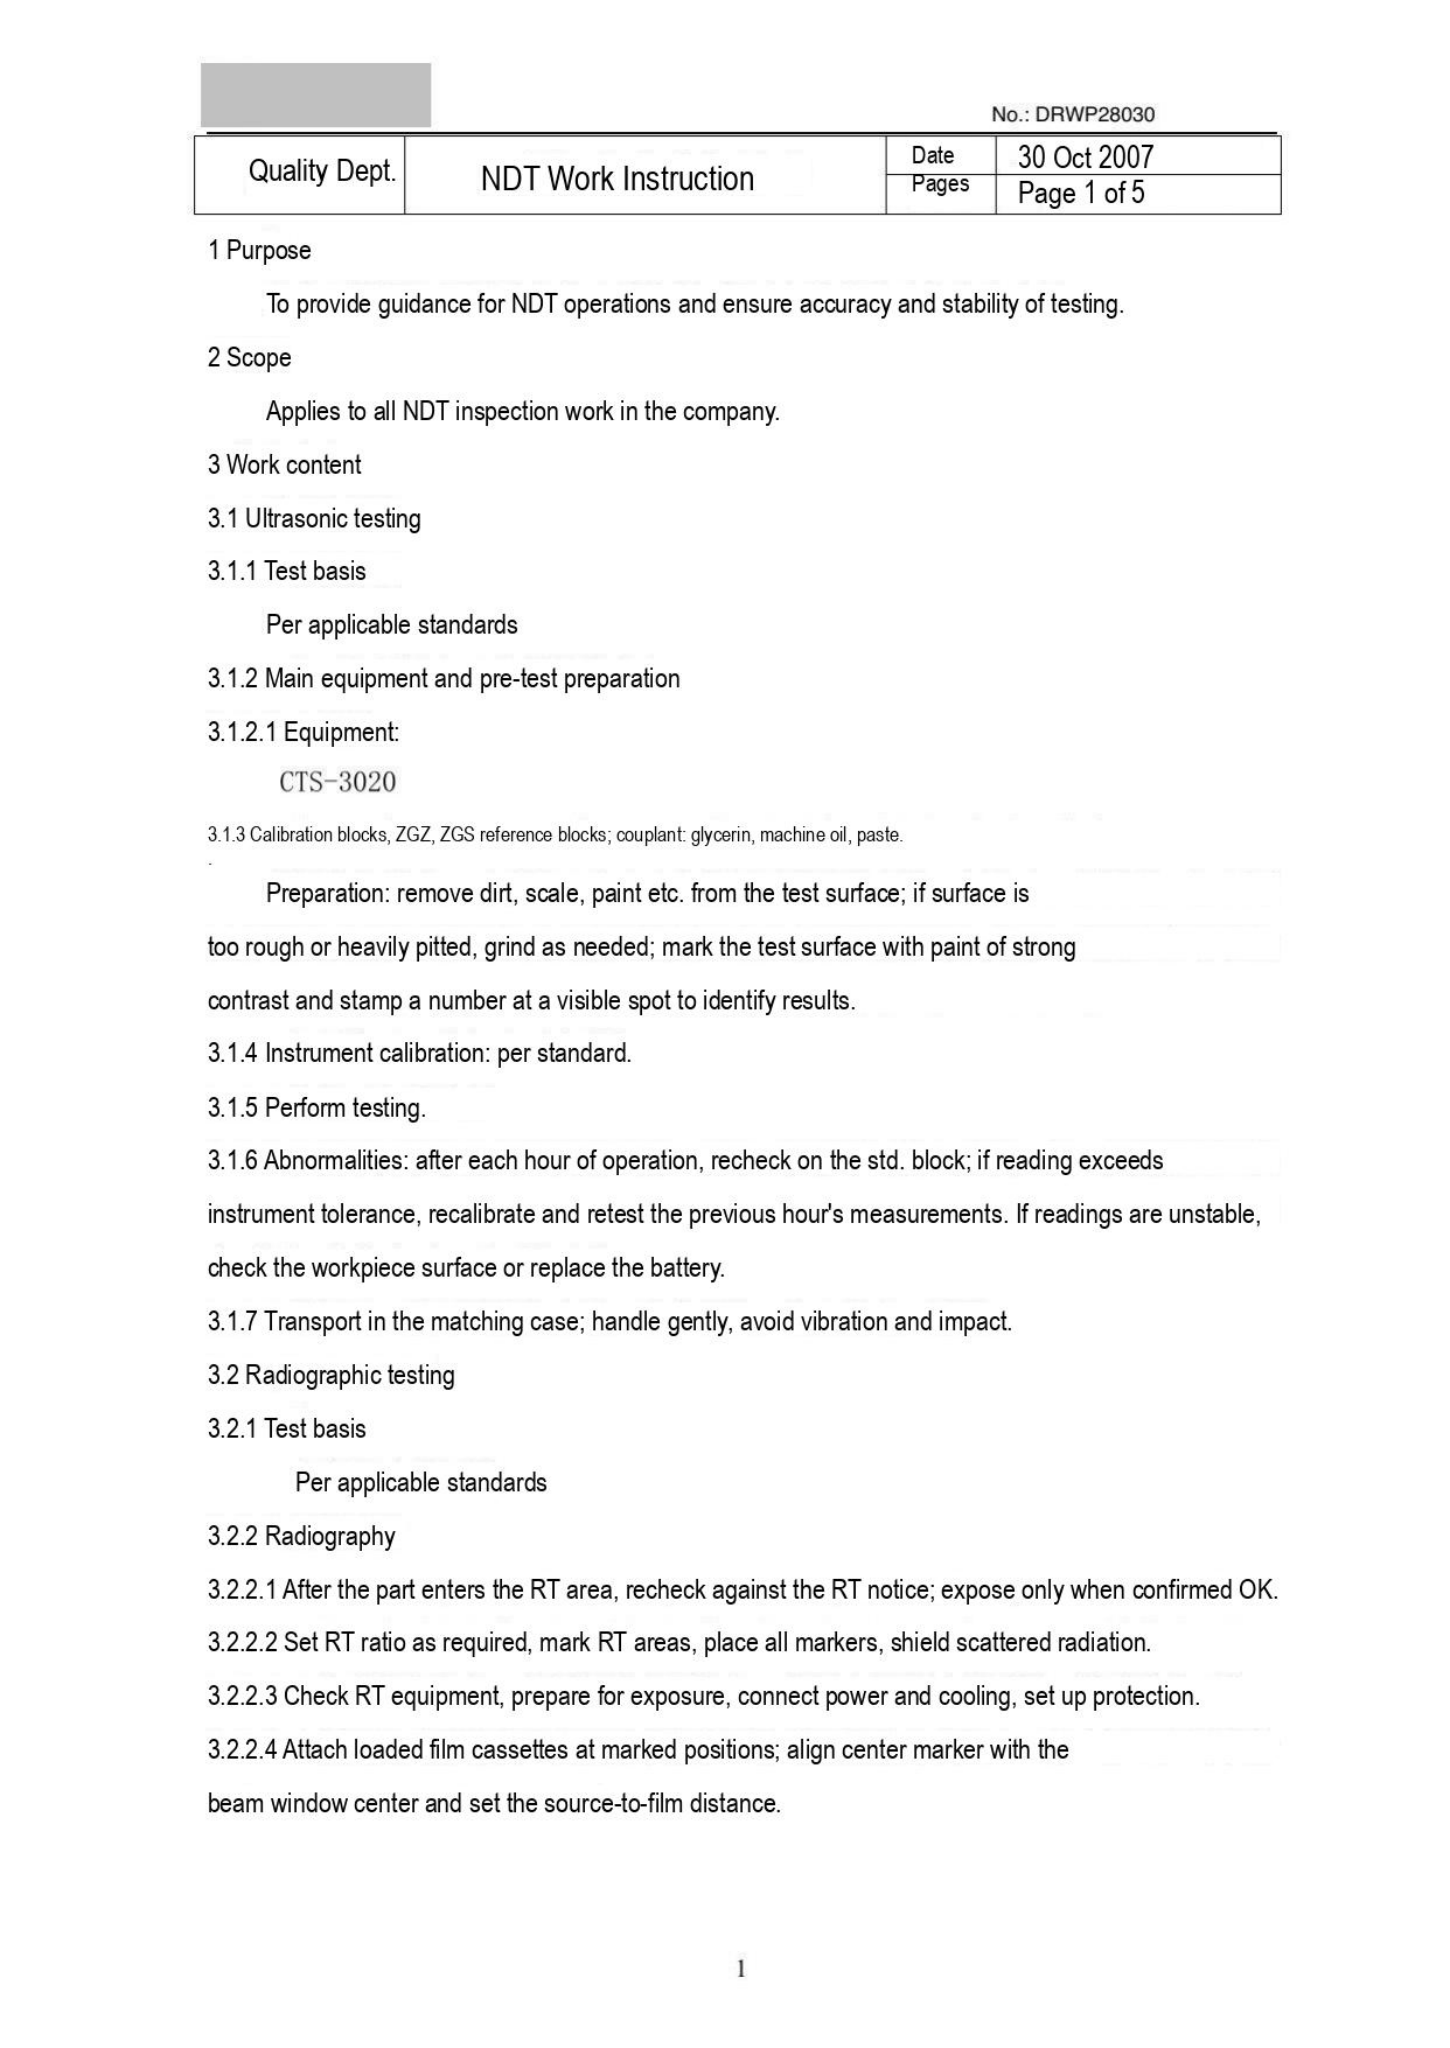No.: DRWP28030

| Quality Dept. | NDT Work Instruction | Date | 30 Oct 2007 |
|---|---|---|---|
| | | Pages | Page 1 of 5 |

1 Purpose

To provide guidance for NDT operations and ensure accuracy and stability of testing.

2 Scope

Applies to all NDT inspection work in the company.

3 Work content

3.1 Ultrasonic testing

3.1.1 Test basis

Per applicable standards

3.1.2 Main equipment and pre-test preparation

3.1.2.1 Equipment:

CTS-3020

3.1.3 Calibration blocks, ZGZ, ZGS reference blocks; couplant: glycerin, machine oil, paste.

Preparation: remove dirt, scale, paint etc. from the test surface; if surface is too rough or heavily pitted, grind as needed; mark the test surface with paint of strong contrast and stamp a number at a visible spot to identify results.

3.1.4 Instrument calibration: per standard.

3.1.5 Perform testing.

3.1.6 Abnormalities: after each hour of operation, recheck on the std. block; if reading exceeds instrument tolerance, recalibrate and retest the previous hour's measurements. If readings are unstable, check the workpiece surface or replace the battery.

3.1.7 Transport in the matching case; handle gently, avoid vibration and impact.

3.2 Radiographic testing

3.2.1 Test basis

Per applicable standards

3.2.2 Radiography

3.2.2.1 After the part enters the RT area, recheck against the RT notice; expose only when confirmed OK.

3.2.2.2 Set RT ratio as required, mark RT areas, place all markers, shield scattered radiation.

3.2.2.3 Check RT equipment, prepare for exposure, connect power and cooling, set up protection.

3.2.2.4 Attach loaded film cassettes at marked positions; align center marker with the beam window center and set the source-to-film distance.

1
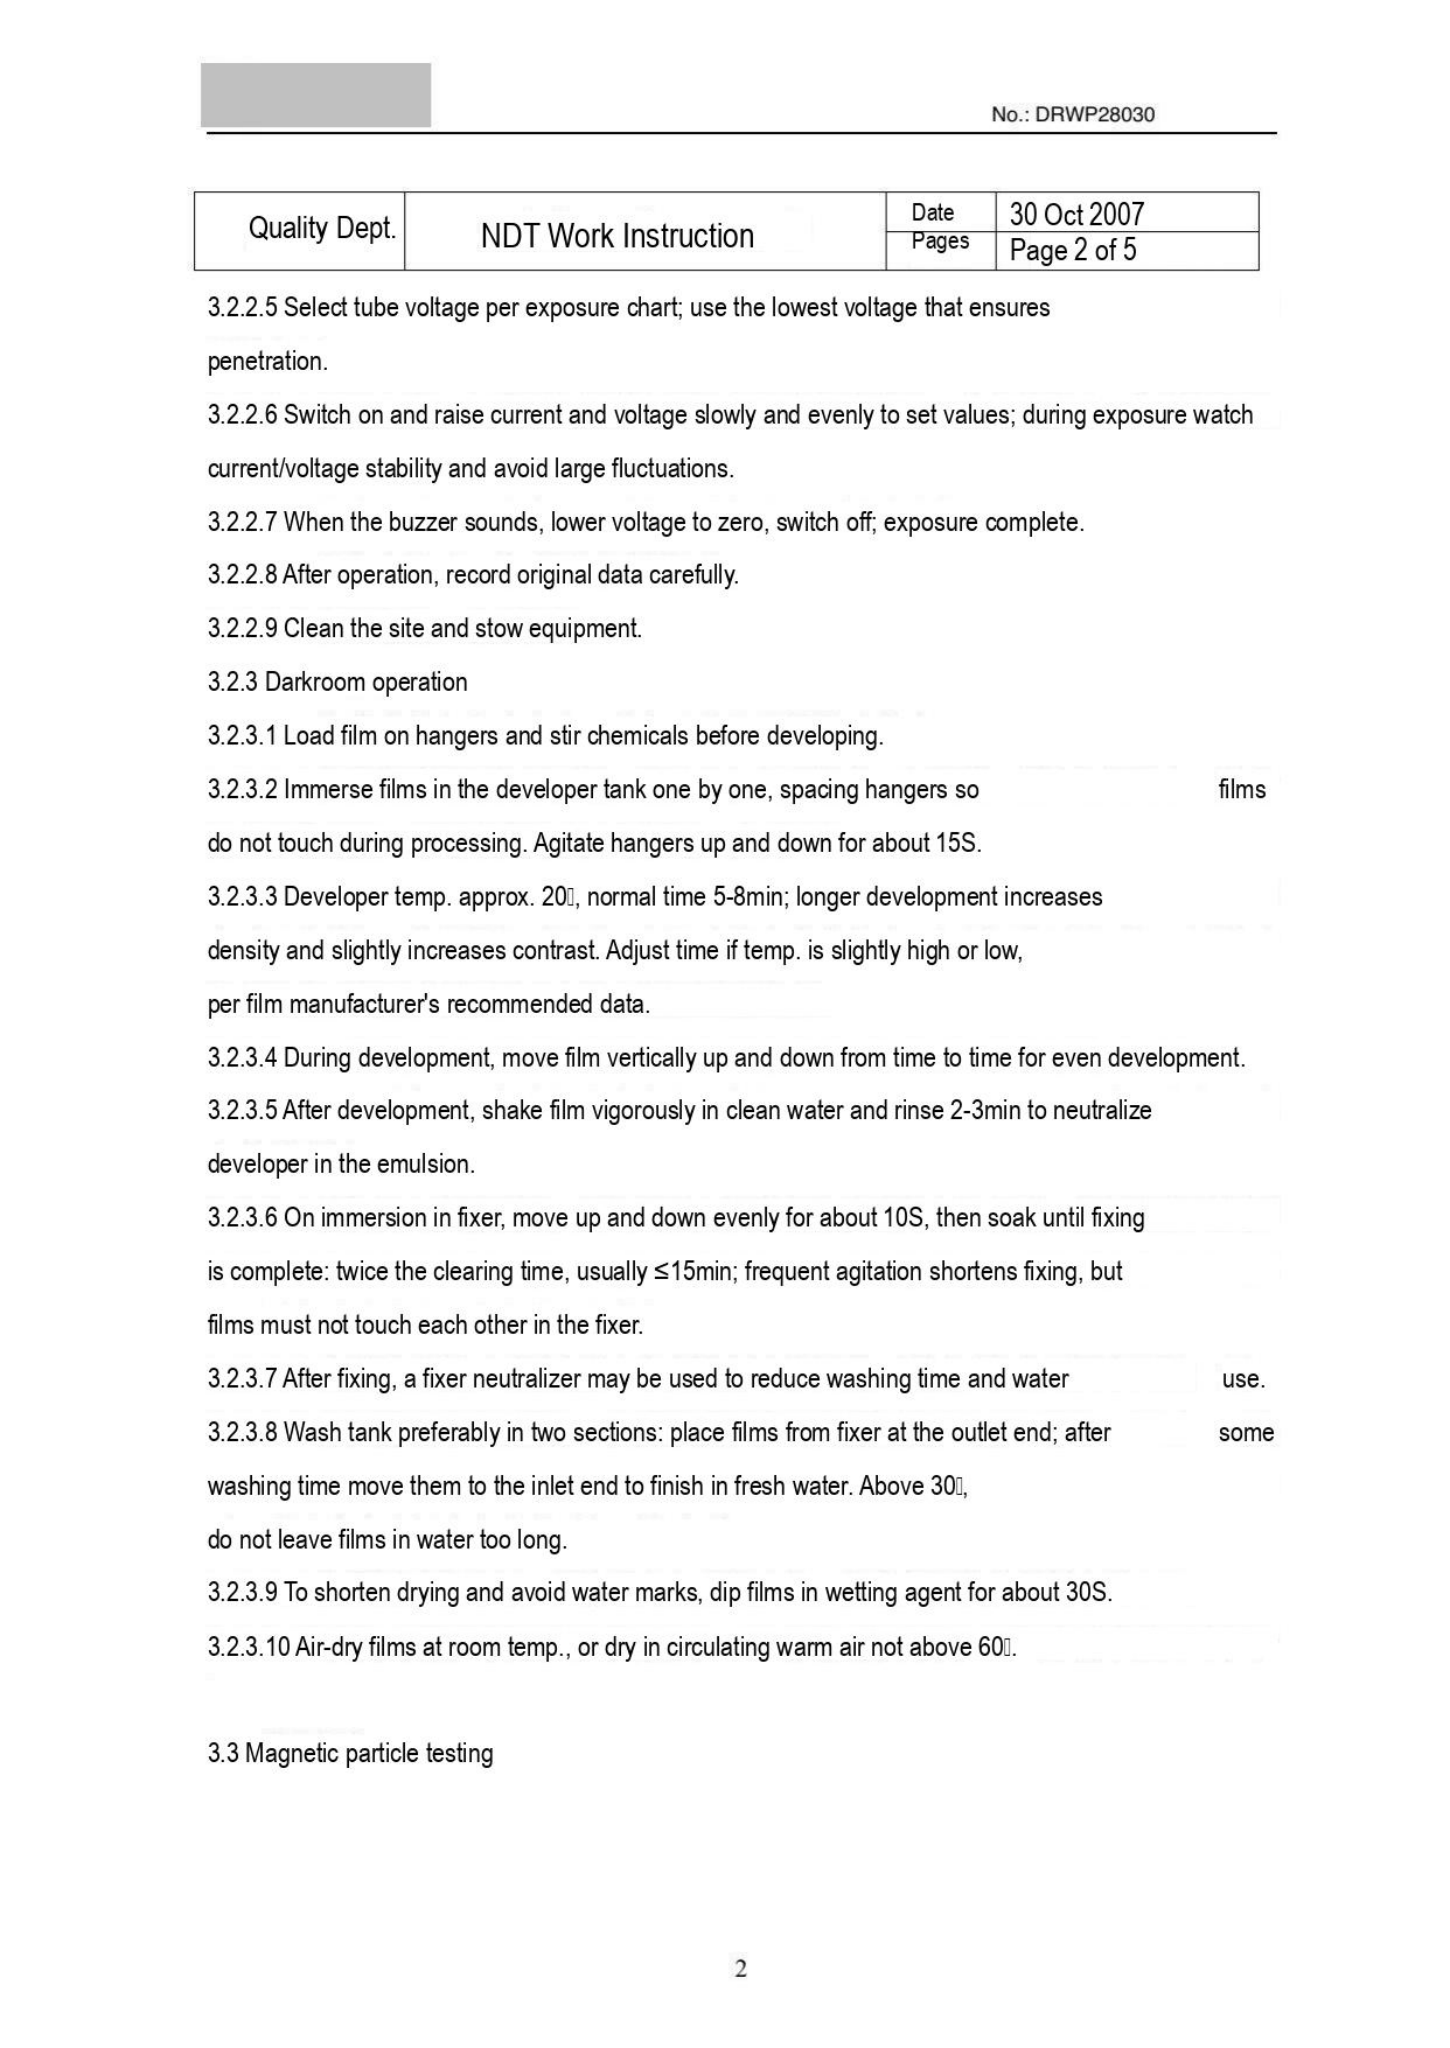No.: DRWP28030

| Quality Dept. | NDT Work Instruction | Date | 30 Oct 2007 |
|---|---|---|---|
| | | Pages | Page 2 of 5 |

3.2.2.5 Select tube voltage per exposure chart; use the lowest voltage that ensures penetration.

3.2.2.6 Switch on and raise current and voltage slowly and evenly to set values; during exposure watch current/voltage stability and avoid large fluctuations.

3.2.2.7 When the buzzer sounds, lower voltage to zero, switch off; exposure complete.

3.2.2.8 After operation, record original data carefully.

3.2.2.9 Clean the site and stow equipment.

3.2.3 Darkroom operation

3.2.3.1 Load film on hangers and stir chemicals before developing.

3.2.3.2 Immerse films in the developer tank one by one, spacing hangers so films do not touch during processing. Agitate hangers up and down for about 15S.

3.2.3.3 Developer temp. approx. 20, normal time 5-8min; longer development increases density and slightly increases contrast. Adjust time if temp. is slightly high or low, per film manufacturer's recommended data.

3.2.3.4 During development, move film vertically up and down from time to time for even development.

3.2.3.5 After development, shake film vigorously in clean water and rinse 2-3min to neutralize developer in the emulsion.

3.2.3.6 On immersion in fixer, move up and down evenly for about 10S, then soak until fixing is complete: twice the clearing time, usually ≤15min; frequent agitation shortens fixing, but films must not touch each other in the fixer.

3.2.3.7 After fixing, a fixer neutralizer may be used to reduce washing time and water use.

3.2.3.8 Wash tank preferably in two sections: place films from fixer at the outlet end; after some washing time move them to the inlet end to finish in fresh water. Above 30, do not leave films in water too long.

3.2.3.9 To shorten drying and avoid water marks, dip films in wetting agent for about 30S.

3.2.3.10 Air-dry films at room temp., or dry in circulating warm air not above 60.

3.3 Magnetic particle testing

2
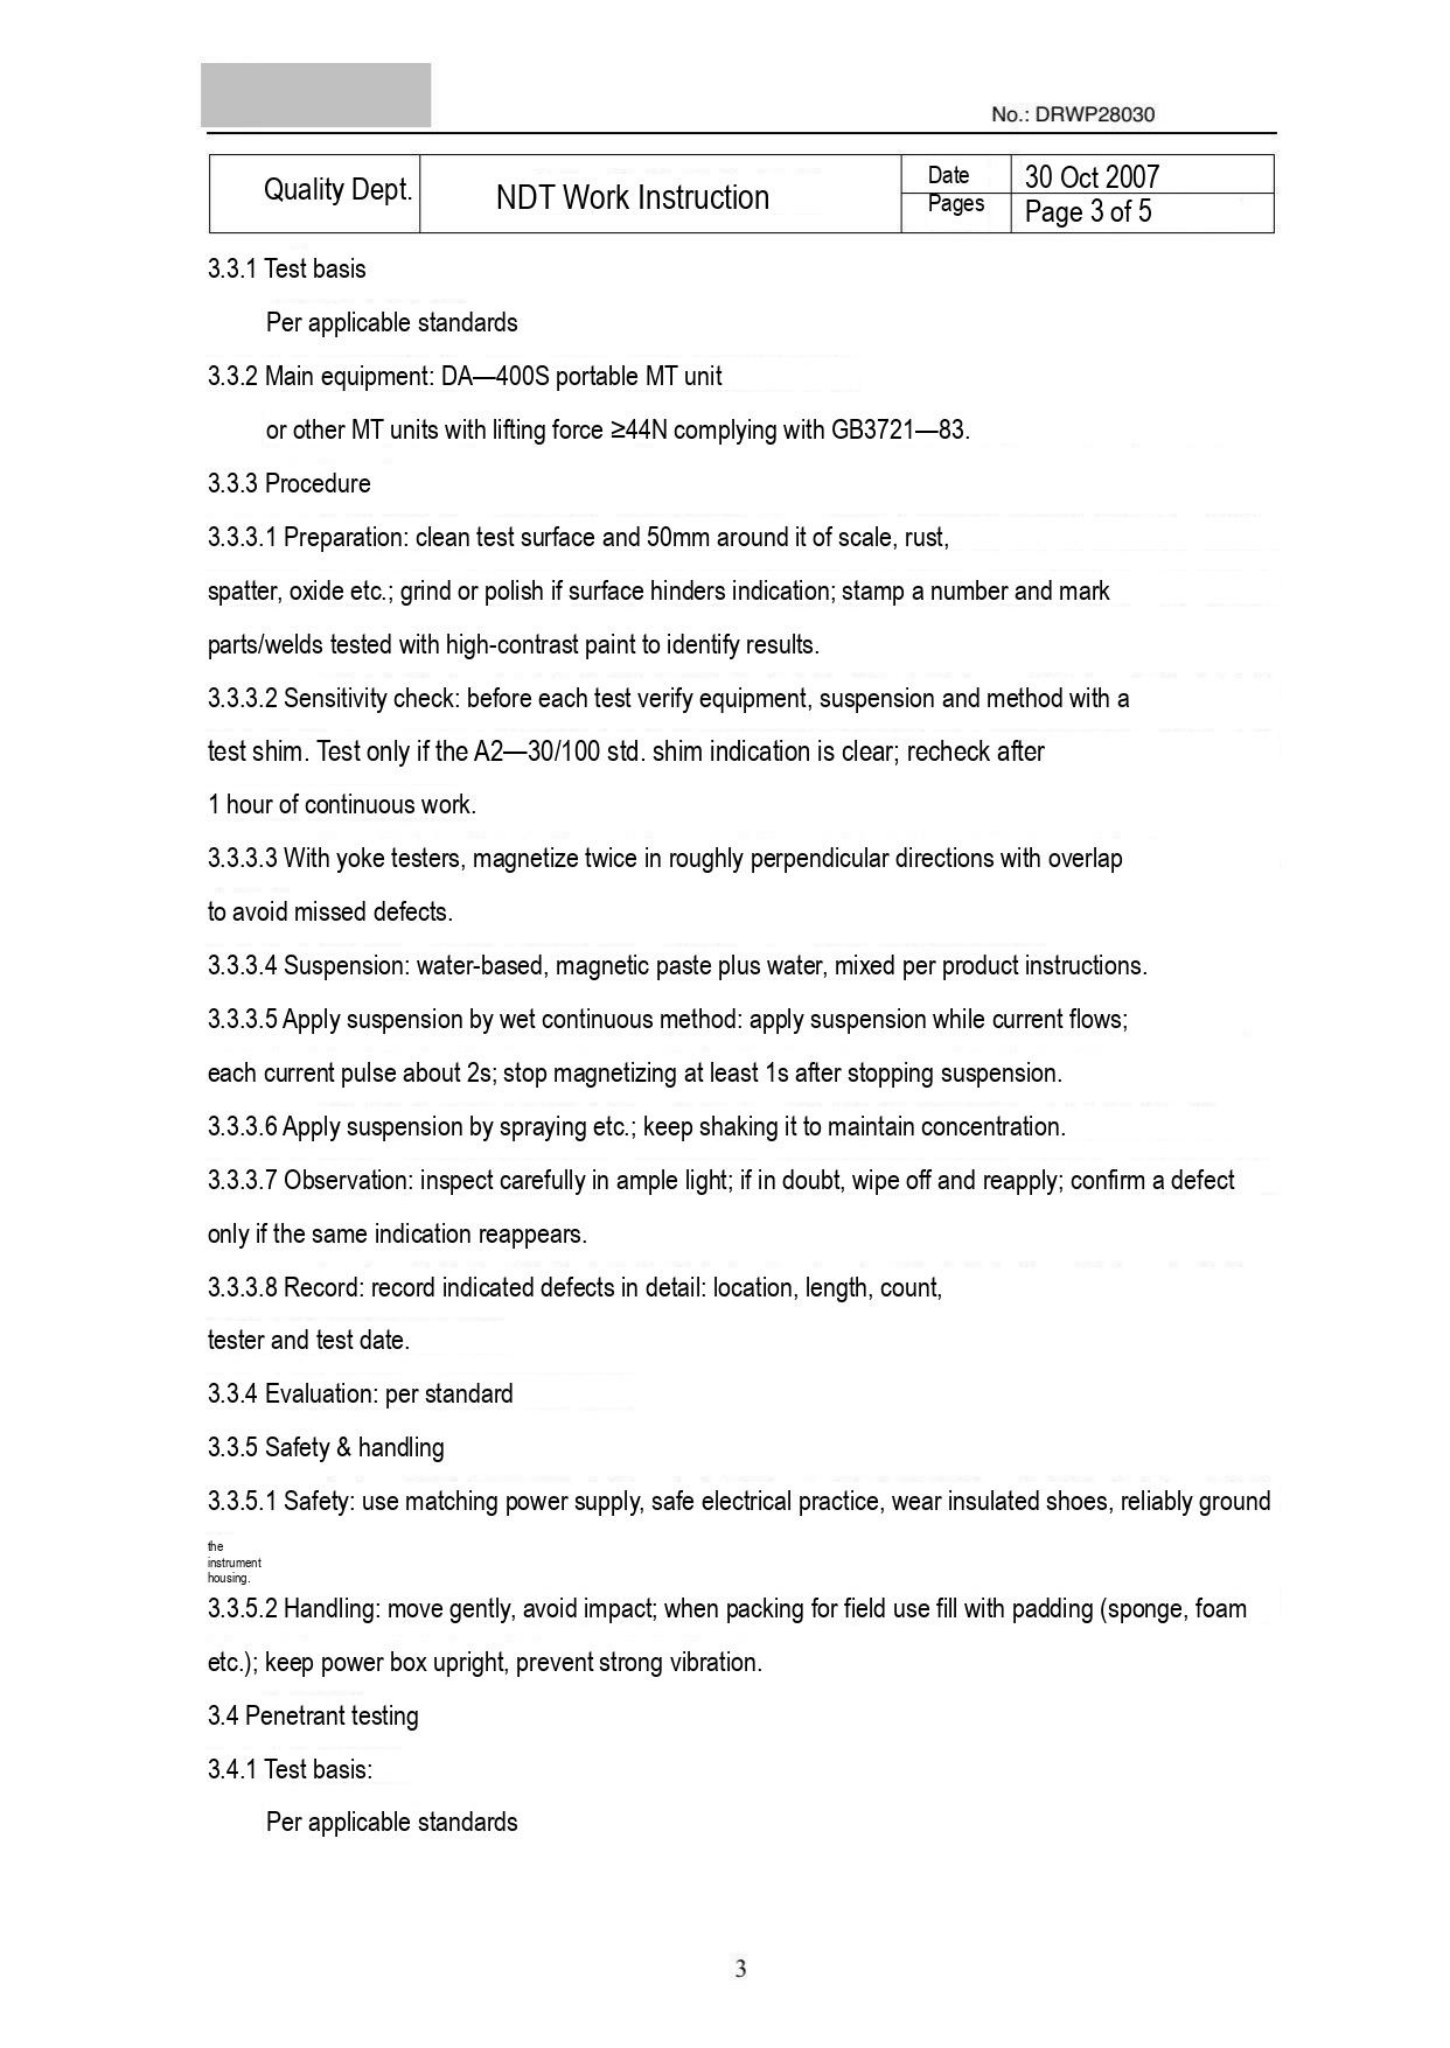No.: DRWP28030

| Quality Dept. | NDT Work Instruction | Date | 30 Oct 2007 |
|---|---|---|---|
| | | Pages | Page 3 of 5 |

3.3.1 Test basis

Per applicable standards

3.3.2 Main equipment: DA—400S portable MT unit

or other MT units with lifting force ≥44N complying with GB3721—83.

3.3.3 Procedure

3.3.3.1 Preparation: clean test surface and 50mm around it of scale, rust, spatter, oxide etc.; grind or polish if surface hinders indication; stamp a number and mark parts/welds tested with high-contrast paint to identify results.

3.3.3.2 Sensitivity check: before each test verify equipment, suspension and method with a test shim. Test only if the A2—30/100 std. shim indication is clear; recheck after 1 hour of continuous work.

3.3.3.3 With yoke testers, magnetize twice in roughly perpendicular directions with overlap to avoid missed defects.

3.3.3.4 Suspension: water-based, magnetic paste plus water, mixed per product instructions.

3.3.3.5 Apply suspension by wet continuous method: apply suspension while current flows; each current pulse about 2s; stop magnetizing at least 1s after stopping suspension.

3.3.3.6 Apply suspension by spraying etc.; keep shaking it to maintain concentration.

3.3.3.7 Observation: inspect carefully in ample light; if in doubt, wipe off and reapply; confirm a defect only if the same indication reappears.

3.3.3.8 Record: record indicated defects in detail: location, length, count, tester and test date.

3.3.4 Evaluation: per standard

3.3.5 Safety & handling

3.3.5.1 Safety: use matching power supply, safe electrical practice, wear insulated shoes, reliably ground the instrument housing.

3.3.5.2 Handling: move gently, avoid impact; when packing for field use fill with padding (sponge, foam etc.); keep power box upright, prevent strong vibration.

3.4 Penetrant testing

3.4.1 Test basis:

Per applicable standards

3
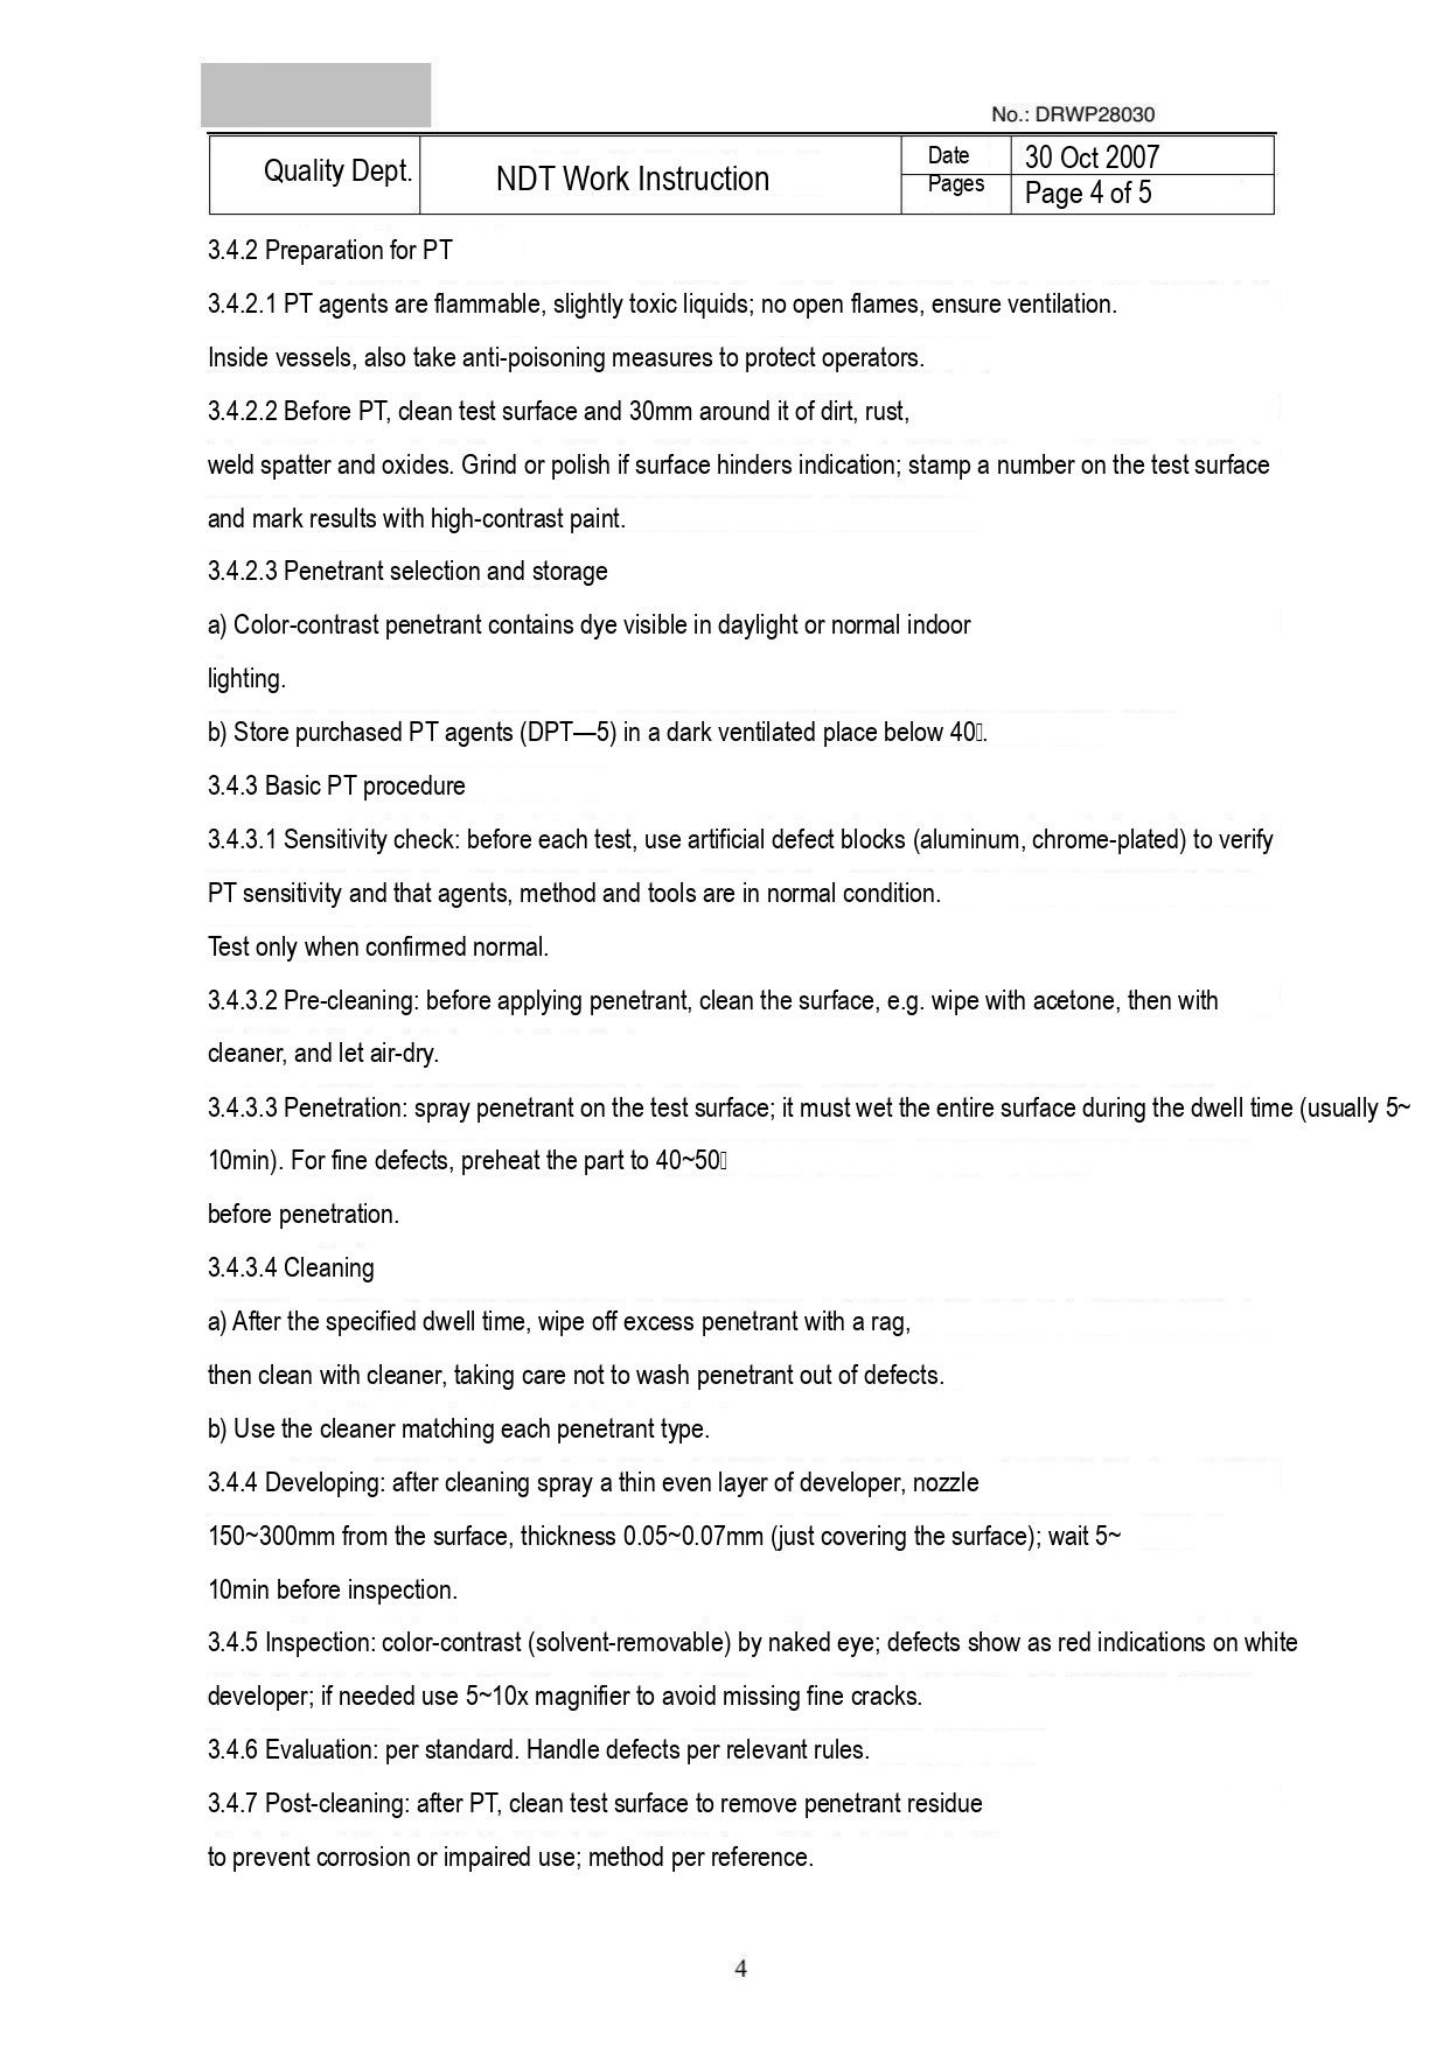No.: DRWP28030

| Quality Dept. | NDT Work Instruction | Date | 30 Oct 2007 |
|---|---|---|---|
| | | Pages | Page 4 of 5 |

3.4.2 Preparation for PT

3.4.2.1 PT agents are flammable, slightly toxic liquids; no open flames, ensure ventilation.

Inside vessels, also take anti-poisoning measures to protect operators.

3.4.2.2 Before PT, clean test surface and 30mm around it of dirt, rust,

weld spatter and oxides. Grind or polish if surface hinders indication; stamp a number on the test surface

and mark results with high-contrast paint.

3.4.2.3 Penetrant selection and storage

a) Color-contrast penetrant contains dye visible in daylight or normal indoor

lighting.

b) Store purchased PT agents (DPT—5) in a dark ventilated place below 40.

3.4.3 Basic PT procedure

3.4.3.1 Sensitivity check: before each test, use artificial defect blocks (aluminum, chrome-plated) to verify

PT sensitivity and that agents, method and tools are in normal condition.

Test only when confirmed normal.

3.4.3.2 Pre-cleaning: before applying penetrant, clean the surface, e.g. wipe with acetone, then with

cleaner, and let air-dry.

3.4.3.3 Penetration: spray penetrant on the test surface; it must wet the entire surface during the dwell time (usually 5~

10min). For fine defects, preheat the part to 40~50

before penetration.

3.4.3.4 Cleaning

a) After the specified dwell time, wipe off excess penetrant with a rag,

then clean with cleaner, taking care not to wash penetrant out of defects.

b) Use the cleaner matching each penetrant type.

3.4.4 Developing: after cleaning spray a thin even layer of developer, nozzle

150~300mm from the surface, thickness 0.05~0.07mm (just covering the surface); wait 5~

10min before inspection.

3.4.5 Inspection: color-contrast (solvent-removable) by naked eye; defects show as red indications on white

developer; if needed use 5~10x magnifier to avoid missing fine cracks.

3.4.6 Evaluation: per standard. Handle defects per relevant rules.

3.4.7 Post-cleaning: after PT, clean test surface to remove penetrant residue

to prevent corrosion or impaired use; method per reference.

4
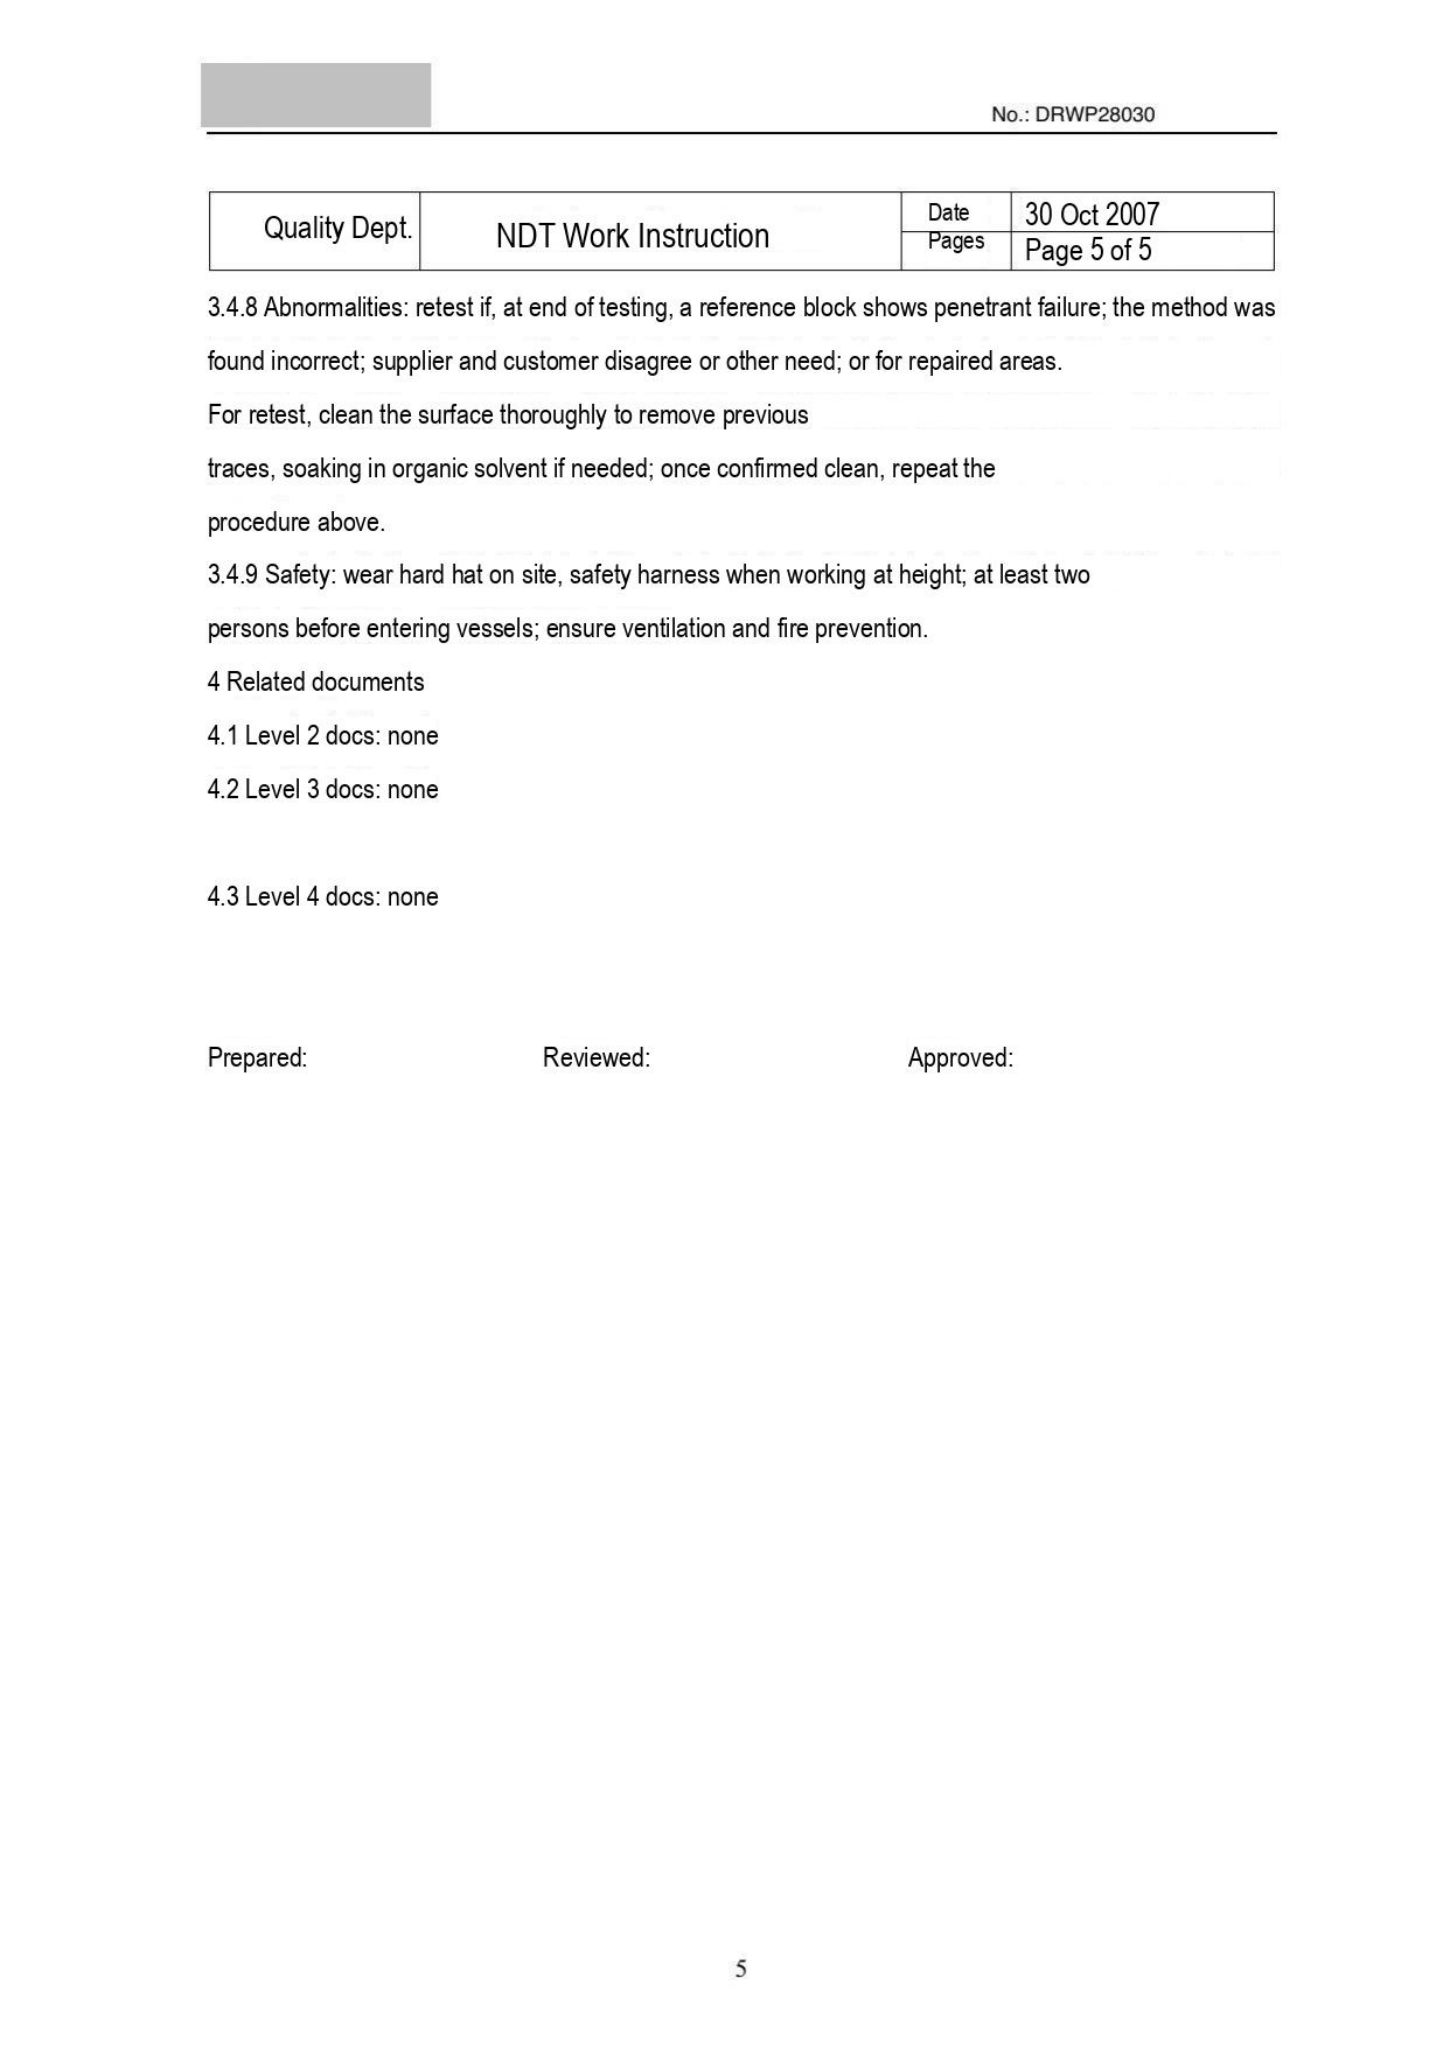No.: DRWP28030

| Quality Dept. | NDT Work Instruction | Date | 30 Oct 2007 |
|---|---|---|---|
| | | Pages | Page 5 of 5 |

3.4.8 Abnormalities: retest if, at end of testing, a reference block shows penetrant failure; the method was found incorrect; supplier and customer disagree or other need; or for repaired areas.

For retest, clean the surface thoroughly to remove previous

traces, soaking in organic solvent if needed; once confirmed clean, repeat the

procedure above.

3.4.9 Safety: wear hard hat on site, safety harness when working at height; at least two

persons before entering vessels; ensure ventilation and fire prevention.

4 Related documents

4.1 Level 2 docs: none

4.2 Level 3 docs: none

4.3 Level 4 docs: none

Prepared: Reviewed: Approved:

5